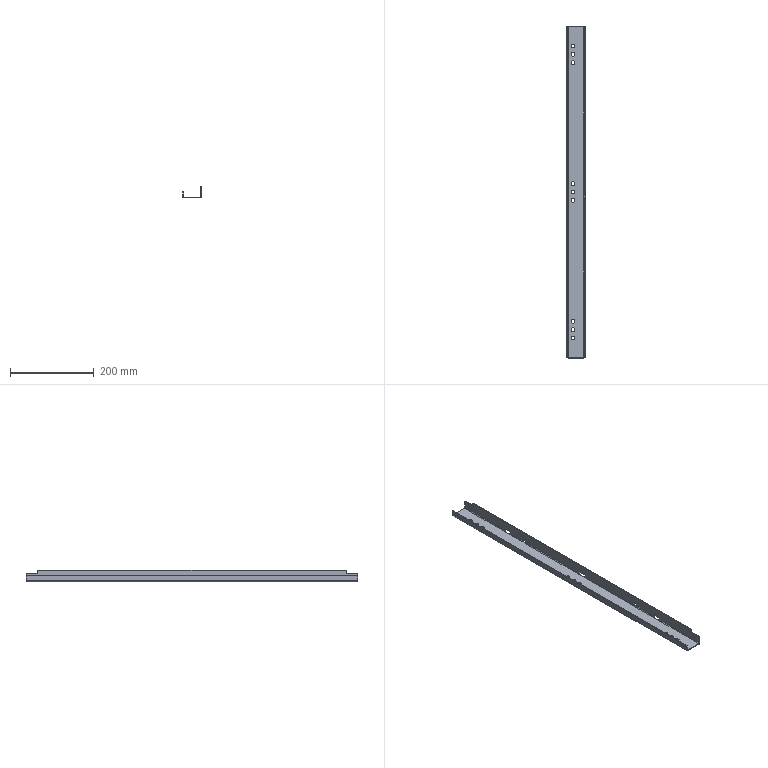Part | STEP file | Middle door gasket strip vertical (hinge) modified | 1 solid | 104 faces | box 44.5 x 791 x 28.5 mm | volume 125821 mm3 | plane 70 | cylinder 34 | commonest cylinder face diameters 9 x18 3 x8 7 x8